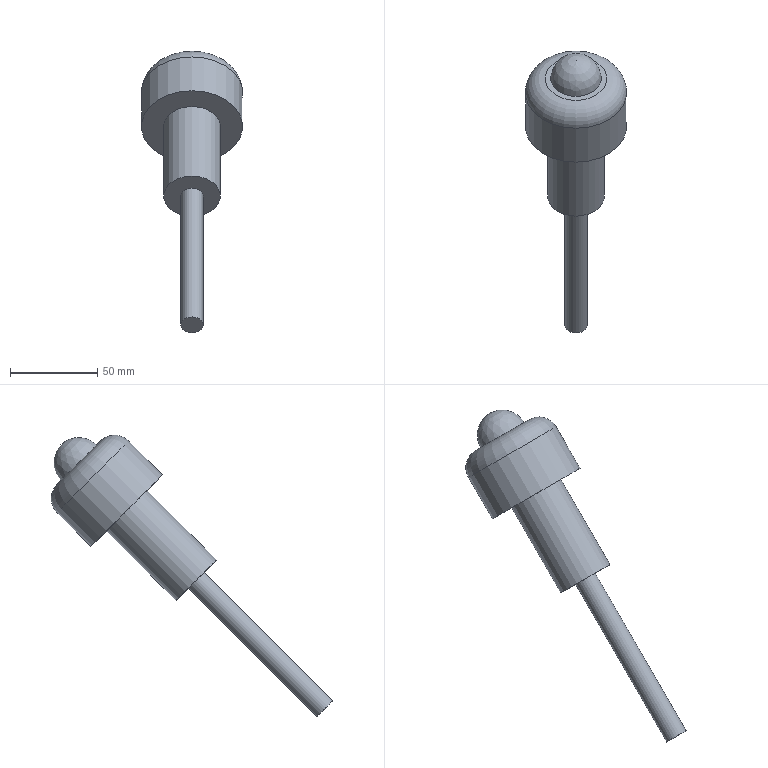Part | NX | features DATUM_CSYS 2, Delete Body 2, LINKED_BODY 2, BLEND 1, DATUM_PLANE 1, SCALE 1, SKETCH 1, SWP104 1 | 1 solid | 9 faces | box 57.861 x 160.996 x 160.996 mm | volume 163265 mm3 | plane 4 | cylinder 3 | sphere 1 | torus 1 | commonest cylinder face diameters 12.834 x1 32.439 x1 57.861 x1
STEP:
#1=CARTESIAN_POINT('',(7.25,2539.64,-794.033));
#2=VERTEX_POINT('',#1);
#3=CARTESIAN_POINT('',(7.25,2544.177,-798.57));
#4=DIRECTION('',(0.,0.7071,0.7071));
#5=DIRECTION('',(0.,-0.7071,0.7071));
#6=AXIS2_PLACEMENT_3D('',#3,#4,#5);
#7=CIRCLE('',#6,6.417);
#8=EDGE_CURVE('',#2,#2,#7,.T.);
#9=ORIENTED_EDGE('',*,*,#8,.F.);
#10=EDGE_LOOP('',(#9));
#11=FACE_BOUND('',#10,.T.);
#12=CARTESIAN_POINT('',(7.25,2544.177,-798.57));
#13=DIRECTION('',(0.,0.7071,0.7071));
#14=DIRECTION('',(0.,-0.7071,0.7071));
#15=AXIS2_PLACEMENT_3D('',#12,#13,#14);
#16=PLANE('',#15);
#17=ADVANCED_FACE('',(#11),#16,.F.);
#18=ORIENTED_EDGE('',*,*,#8,.T.);
#19=EDGE_LOOP('',(#18));
#20=FACE_BOUND('',#19,.T.);
#21=CARTESIAN_POINT('',(7.25,2613.223,-720.45));
#22=VERTEX_POINT('',#21);
#23=CARTESIAN_POINT('',(7.25,2617.76,-724.987));
#24=DIRECTION('',(0.,0.7071,0.7071));
#25=DIRECTION('',(0.,-0.7071,0.7071));
#26=AXIS2_PLACEMENT_3D('',#23,#24,#25);
#27=CIRCLE('',#26,6.417);
#28=EDGE_CURVE('',#22,#22,#27,.T.);
#29=ORIENTED_EDGE('',*,*,#28,.F.);
#30=EDGE_LOOP('',(#29));
#31=FACE_BOUND('',#30,.T.);
#32=CARTESIAN_POINT('',(7.25,2695.043,-647.705));
#33=DIRECTION('',(0.,0.7071,0.7071));
#34=DIRECTION('',(0.,-0.7071,0.7071));
#35=AXIS2_PLACEMENT_3D('',#32,#33,#34);
#36=CYLINDRICAL_SURFACE('',#35,6.417);
#37=ADVANCED_FACE('',(#20,#31),#36,.T.);
#38=ORIENTED_EDGE('',*,*,#28,.T.);
#39=EDGE_LOOP('',(#38));
#40=FACE_BOUND('',#39,.T.);
#41=CARTESIAN_POINT('',(7.25,2606.292,-713.518));
#42=VERTEX_POINT('',#41);
#43=CARTESIAN_POINT('',(7.25,2617.76,-724.987));
#44=DIRECTION('',(0.,0.7071,0.7071));
#45=DIRECTION('',(0.,-0.7071,0.7071));
#46=AXIS2_PLACEMENT_3D('',#43,#44,#45);
#47=CIRCLE('',#46,16.219);
#48=EDGE_CURVE('',#42,#42,#47,.T.);
#49=ORIENTED_EDGE('',*,*,#48,.F.);
#50=EDGE_LOOP('',(#49));
#51=FACE_BOUND('',#50,.T.);
#52=CARTESIAN_POINT('',(7.25,2606.292,-713.518));
#53=DIRECTION('',(0.,-0.7071,-0.7071));
#54=DIRECTION('',(0.,0.7071,-0.7071));
#55=AXIS2_PLACEMENT_3D('',#52,#53,#54);
#56=PLANE('',#55);
#57=ADVANCED_FACE('',(#40,#51),#56,.T.);
#58=ORIENTED_EDGE('',*,*,#48,.T.);
#59=EDGE_LOOP('',(#58));
#60=FACE_BOUND('',#59,.T.);
#61=CARTESIAN_POINT('',(7.25,2646.066,-673.743));
#62=VERTEX_POINT('',#61);
#63=CARTESIAN_POINT('',(7.25,2657.535,-685.212));
#64=DIRECTION('',(0.,0.7071,0.7071));
#65=DIRECTION('',(0.,-0.7071,0.7071));
#66=AXIS2_PLACEMENT_3D('',#63,#64,#65);
#67=CIRCLE('',#66,16.219);
#68=EDGE_CURVE('',#62,#62,#67,.T.);
#69=ORIENTED_EDGE('',*,*,#68,.F.);
#70=EDGE_LOOP('',(#69));
#71=FACE_BOUND('',#70,.T.);
#72=CARTESIAN_POINT('',(7.25,2695.043,-647.705));
#73=DIRECTION('',(0.,0.7071,0.7071));
#74=DIRECTION('',(0.,-0.7071,0.7071));
#75=AXIS2_PLACEMENT_3D('',#72,#73,#74);
#76=CYLINDRICAL_SURFACE('',#75,16.219);
#77=ADVANCED_FACE('',(#60,#71),#76,.T.);
#78=ORIENTED_EDGE('',*,*,#68,.T.);
#79=EDGE_LOOP('',(#78));
#80=FACE_BOUND('',#79,.T.);
#81=CARTESIAN_POINT('',(7.25,2637.078,-664.755));
#82=VERTEX_POINT('',#81);
#83=CARTESIAN_POINT('',(7.25,2657.535,-685.212));
#84=DIRECTION('',(0.,0.7071,0.7071));
#85=DIRECTION('',(0.,-0.7071,0.7071));
#86=AXIS2_PLACEMENT_3D('',#83,#84,#85);
#87=CIRCLE('',#86,28.931);
#88=EDGE_CURVE('',#82,#82,#87,.T.);
#89=ORIENTED_EDGE('',*,*,#88,.F.);
#90=EDGE_LOOP('',(#89));
#91=FACE_BOUND('',#90,.T.);
#92=CARTESIAN_POINT('',(7.25,2637.078,-664.755));
#93=DIRECTION('',(0.,-0.7071,-0.7071));
#94=DIRECTION('',(0.,0.7071,-0.7071));
#95=AXIS2_PLACEMENT_3D('',#92,#93,#94);
#96=PLANE('',#95);
#97=ADVANCED_FACE('',(#80,#91),#96,.T.);
#98=CARTESIAN_POINT('',(7.25,2656.426,-645.407));
#99=VERTEX_POINT('',#98);
#100=CARTESIAN_POINT('',(7.25,2676.883,-665.864));
#101=DIRECTION('',(0.,0.7071,0.7071));
#102=DIRECTION('',(0.,-0.7071,0.7071));
#103=AXIS2_PLACEMENT_3D('',#100,#101,#102);
#104=CIRCLE('',#103,28.931);
#105=EDGE_CURVE('',#99,#99,#104,.F.);
#106=ORIENTED_EDGE('',*,*,#105,.T.);
#107=EDGE_LOOP('',(#106));
#108=FACE_BOUND('',#107,.T.);
#109=ORIENTED_EDGE('',*,*,#88,.T.);
#110=EDGE_LOOP('',(#109));
#111=FACE_BOUND('',#110,.T.);
#112=CARTESIAN_POINT('',(7.25,2695.043,-647.705));
#113=DIRECTION('',(0.,0.7071,0.7071));
#114=DIRECTION('',(0.,-0.7071,0.7071));
#115=AXIS2_PLACEMENT_3D('',#112,#113,#114);
#116=CYLINDRICAL_SURFACE('',#115,28.931);
#117=ADVANCED_FACE('',(#108,#111),#116,.T.);
#118=CARTESIAN_POINT('',(7.25,2672.336,-645.407));
#119=VERTEX_POINT('',#118);
#120=CARTESIAN_POINT('',(7.25,2684.838,-657.909));
#121=DIRECTION('',(0.,0.7071,0.7071));
#122=DIRECTION('',(0.,-0.7071,0.7071));
#123=AXIS2_PLACEMENT_3D('',#120,#121,#122);
#124=CIRCLE('',#123,17.681);
#125=EDGE_CURVE('',#119,#119,#124,.T.);
#126=ORIENTED_EDGE('',*,*,#125,.T.);
#127=EDGE_LOOP('',(#126));
#128=FACE_BOUND('',#127,.T.);
#129=CARTESIAN_POINT('',(7.25,2674.634,-647.705));
#130=VERTEX_POINT('',#129);
#131=CARTESIAN_POINT('',(7.25,2684.838,-657.909));
#132=DIRECTION('',(0.,0.7071,0.7071));
#133=DIRECTION('',(0.,-0.7071,0.7071));
#134=AXIS2_PLACEMENT_3D('',#131,#132,#133);
#135=CIRCLE('',#134,14.431);
#136=EDGE_CURVE('',#130,#130,#135,.T.);
#137=ORIENTED_EDGE('',*,*,#136,.F.);
#138=EDGE_LOOP('',(#137));
#139=FACE_BOUND('',#138,.T.);
#140=CARTESIAN_POINT('',(7.25,2674.634,-647.705));
#141=DIRECTION('',(0.,0.7071,0.7071));
#142=DIRECTION('',(0.,-0.7071,0.7071));
#143=AXIS2_PLACEMENT_3D('',#140,#141,#142);
#144=PLANE('',#143);
#145=ADVANCED_FACE('',(#128,#139),#144,.T.);
#146=ORIENTED_EDGE('',*,*,#136,.T.);
#147=EDGE_LOOP('',(#146));
#148=FACE_BOUND('',#147,.T.);
#149=CARTESIAN_POINT('',(7.25,2684.838,-657.909));
#150=DIRECTION('',(0.,0.7071,0.7071));
#151=DIRECTION('',(0.,-0.7071,0.7071));
#152=AXIS2_PLACEMENT_3D('',#149,#150,#151);
#153=SPHERICAL_SURFACE('',#152,14.431);
#154=ADVANCED_FACE('',(#148),#153,.T.);
#155=ORIENTED_EDGE('',*,*,#105,.F.);
#156=EDGE_LOOP('',(#155));
#157=FACE_BOUND('',#156,.T.);
#158=ORIENTED_EDGE('',*,*,#125,.F.);
#159=EDGE_LOOP('',(#158));
#160=FACE_BOUND('',#159,.T.);
#161=CARTESIAN_POINT('',(7.25,2676.883,-665.864));
#162=DIRECTION('',(0.,0.7071,0.7071));
#163=DIRECTION('',(0.,-0.7071,0.7071));
#164=AXIS2_PLACEMENT_3D('',#161,#162,#163);
#165=TOROIDAL_SURFACE('',#164,17.681,11.25);
#166=ADVANCED_FACE('',(#157,#160),#165,.T.);
#167=CLOSED_SHELL('',(#17,#37,#57,#77,#97,#117,#145,#154,#166));
#168=MANIFOLD_SOLID_BREP('',#167);
#169=(LENGTH_UNIT()NAMED_UNIT(*)SI_UNIT(.MILLI.,.METRE.));
#170=UNCERTAINTY_MEASURE_WITH_UNIT(LENGTH_MEASURE(0.00001),#169,'','');
#171=(NAMED_UNIT(*)PLANE_ANGLE_UNIT()SI_UNIT($,.RADIAN.));
#172=(NAMED_UNIT(*)SI_UNIT($,.STERADIAN.)SOLID_ANGLE_UNIT());
#173=(GEOMETRIC_REPRESENTATION_CONTEXT(3)GLOBAL_UNCERTAINTY_ASSIGNED_CONTEXT((#170))GLOBAL_UNIT_ASSIGNED_CONTEXT((#169,#171,#172))REPRESENTATION_CONTEXT('',''));
#174=ADVANCED_BREP_SHAPE_REPRESENTATION('',(#168),#173);